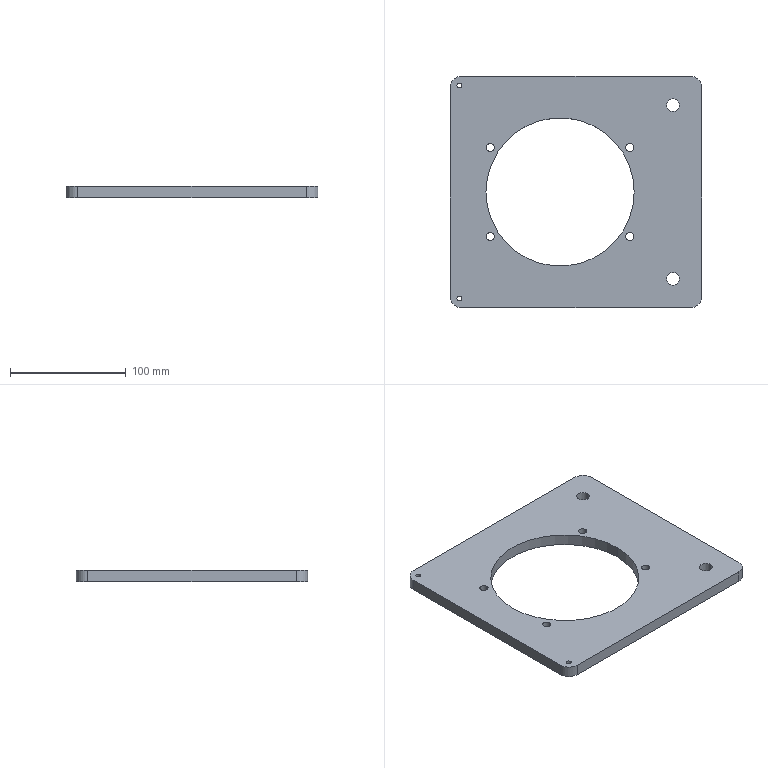Part | SolidWorks | features ICE 3, Cut 2, Extrusion 1, Fillet 1, HoleWzd 1 | 1 solid | 28 faces | box 217.5 x 200 x 10 mm | volume 301745 mm3 | cylinder 22 | plane 6 | commonest cylinder face diameters 7 x8 4.2 x4 11 x4 20 x4 128 x2
STEP:
#1=CARTESIAN_POINT('',(-84.9,92.,0.));
#2=VERTEX_POINT('',#1);
#3=CARTESIAN_POINT('',(-89.1,92.,0.));
#4=VERTEX_POINT('',#3);
#5=CARTESIAN_POINT('',(-87.,92.,0.));
#6=DIRECTION('',(0.,0.,-1.));
#7=DIRECTION('',(-1.,0.,0.));
#8=AXIS2_PLACEMENT_3D('',#5,#6,#7);
#9=CIRCLE('',#8,2.1);
#10=EDGE_CURVE('',#2,#4,#9,.T.);
#11=ORIENTED_EDGE('',*,*,#10,.T.);
#12=CARTESIAN_POINT('',(-89.1,92.,10.));
#13=VERTEX_POINT('',#12);
#14=CARTESIAN_POINT('',(-89.1,92.,10.));
#15=DIRECTION('',(0.,0.,1.));
#16=VECTOR('',#15,1000.);
#17=LINE('',#14,#16);
#18=EDGE_CURVE('',#4,#13,#17,.T.);
#19=ORIENTED_EDGE('',*,*,#18,.T.);
#20=CARTESIAN_POINT('',(-84.9,92.,10.));
#21=VERTEX_POINT('',#20);
#22=CARTESIAN_POINT('',(-87.,92.,10.));
#23=DIRECTION('',(0.,0.,1.));
#24=DIRECTION('',(1.,0.,0.));
#25=AXIS2_PLACEMENT_3D('',#22,#23,#24);
#26=CIRCLE('',#25,2.1);
#27=EDGE_CURVE('',#13,#21,#26,.T.);
#28=ORIENTED_EDGE('',*,*,#27,.T.);
#29=CARTESIAN_POINT('',(-84.9,92.,10.));
#30=DIRECTION('',(0.,0.,1.));
#31=VECTOR('',#30,1000.);
#32=LINE('',#29,#31);
#33=EDGE_CURVE('',#2,#21,#32,.T.);
#34=ORIENTED_EDGE('',*,*,#33,.F.);
#35=EDGE_LOOP('',(#11,#19,#28,#34));
#36=FACE_OUTER_BOUND('',#35,.T.);
#37=CARTESIAN_POINT('',(-87.,92.,10.));
#38=DIRECTION('',(0.,0.,1.));
#39=DIRECTION('',(1.,0.,0.));
#40=AXIS2_PLACEMENT_3D('',#37,#38,#39);
#41=CYLINDRICAL_SURFACE('',#40,2.1);
#42=ADVANCED_FACE('',(#36),#41,.F.);
#43=CARTESIAN_POINT('',(-84.9,-92.,0.));
#44=VERTEX_POINT('',#43);
#45=CARTESIAN_POINT('',(-89.1,-92.,0.));
#46=VERTEX_POINT('',#45);
#47=CARTESIAN_POINT('',(-87.,-92.,0.));
#48=DIRECTION('',(0.,0.,-1.));
#49=DIRECTION('',(-1.,0.,0.));
#50=AXIS2_PLACEMENT_3D('',#47,#48,#49);
#51=CIRCLE('',#50,2.1);
#52=EDGE_CURVE('',#44,#46,#51,.T.);
#53=ORIENTED_EDGE('',*,*,#52,.T.);
#54=CARTESIAN_POINT('',(-89.1,-92.,10.));
#55=VERTEX_POINT('',#54);
#56=CARTESIAN_POINT('',(-89.1,-92.,10.));
#57=DIRECTION('',(0.,0.,1.));
#58=VECTOR('',#57,1000.);
#59=LINE('',#56,#58);
#60=EDGE_CURVE('',#46,#55,#59,.T.);
#61=ORIENTED_EDGE('',*,*,#60,.T.);
#62=CARTESIAN_POINT('',(-84.9,-92.,10.));
#63=VERTEX_POINT('',#62);
#64=CARTESIAN_POINT('',(-87.,-92.,10.));
#65=DIRECTION('',(0.,0.,1.));
#66=DIRECTION('',(1.,0.,0.));
#67=AXIS2_PLACEMENT_3D('',#64,#65,#66);
#68=CIRCLE('',#67,2.1);
#69=EDGE_CURVE('',#55,#63,#68,.T.);
#70=ORIENTED_EDGE('',*,*,#69,.T.);
#71=CARTESIAN_POINT('',(-84.9,-92.,10.));
#72=DIRECTION('',(0.,0.,1.));
#73=VECTOR('',#72,1000.);
#74=LINE('',#71,#73);
#75=EDGE_CURVE('',#44,#63,#74,.T.);
#76=ORIENTED_EDGE('',*,*,#75,.F.);
#77=EDGE_LOOP('',(#53,#61,#70,#76));
#78=FACE_OUTER_BOUND('',#77,.T.);
#79=CARTESIAN_POINT('',(-87.,-92.,10.));
#80=DIRECTION('',(0.,0.,1.));
#81=DIRECTION('',(1.,0.,0.));
#82=AXIS2_PLACEMENT_3D('',#79,#80,#81);
#83=CYLINDRICAL_SURFACE('',#82,2.1);
#84=ADVANCED_FACE('',(#78),#83,.F.);
#85=CARTESIAN_POINT('',(92.,-75.,0.));
#86=VERTEX_POINT('',#85);
#87=CARTESIAN_POINT('',(103.,-75.,0.));
#88=VERTEX_POINT('',#87);
#89=CARTESIAN_POINT('',(97.5,-75.,0.));
#90=DIRECTION('',(0.,0.,1.));
#91=DIRECTION('',(-1.,0.,0.));
#92=AXIS2_PLACEMENT_3D('',#89,#90,#91);
#93=CIRCLE('',#92,5.5);
#94=EDGE_CURVE('',#86,#88,#93,.T.);
#95=ORIENTED_EDGE('',*,*,#94,.F.);
#96=CARTESIAN_POINT('',(92.,-75.,10.));
#97=VERTEX_POINT('',#96);
#98=CARTESIAN_POINT('',(92.,-75.,0.));
#99=DIRECTION('',(0.,0.,1.));
#100=VECTOR('',#99,1000.);
#101=LINE('',#98,#100);
#102=EDGE_CURVE('',#86,#97,#101,.T.);
#103=ORIENTED_EDGE('',*,*,#102,.T.);
#104=CARTESIAN_POINT('',(103.,-75.,10.));
#105=VERTEX_POINT('',#104);
#106=CARTESIAN_POINT('',(97.5,-75.,10.));
#107=DIRECTION('',(0.,0.,1.));
#108=DIRECTION('',(-1.,0.,0.));
#109=AXIS2_PLACEMENT_3D('',#106,#107,#108);
#110=CIRCLE('',#109,5.5);
#111=EDGE_CURVE('',#97,#105,#110,.T.);
#112=ORIENTED_EDGE('',*,*,#111,.T.);
#113=CARTESIAN_POINT('',(103.,-75.,0.));
#114=DIRECTION('',(0.,0.,1.));
#115=VECTOR('',#114,1000.);
#116=LINE('',#113,#115);
#117=EDGE_CURVE('',#88,#105,#116,.T.);
#118=ORIENTED_EDGE('',*,*,#117,.F.);
#119=EDGE_LOOP('',(#95,#103,#112,#118));
#120=FACE_OUTER_BOUND('',#119,.T.);
#121=CARTESIAN_POINT('',(97.5,-75.,0.));
#122=DIRECTION('',(0.,0.,1.));
#123=DIRECTION('',(1.,0.,0.));
#124=AXIS2_PLACEMENT_3D('',#121,#122,#123);
#125=CYLINDRICAL_SURFACE('',#124,5.5);
#126=ADVANCED_FACE('',(#120),#125,.F.);
#127=CARTESIAN_POINT('',(92.,75.,0.));
#128=VERTEX_POINT('',#127);
#129=CARTESIAN_POINT('',(103.,75.,0.));
#130=VERTEX_POINT('',#129);
#131=CARTESIAN_POINT('',(97.5,75.,0.));
#132=DIRECTION('',(0.,0.,1.));
#133=DIRECTION('',(1.,0.,0.));
#134=AXIS2_PLACEMENT_3D('',#131,#132,#133);
#135=CIRCLE('',#134,5.5);
#136=EDGE_CURVE('',#128,#130,#135,.T.);
#137=ORIENTED_EDGE('',*,*,#136,.F.);
#138=CARTESIAN_POINT('',(92.,75.,10.));
#139=VERTEX_POINT('',#138);
#140=CARTESIAN_POINT('',(92.,75.,0.));
#141=DIRECTION('',(0.,0.,1.));
#142=VECTOR('',#141,1000.);
#143=LINE('',#140,#142);
#144=EDGE_CURVE('',#128,#139,#143,.T.);
#145=ORIENTED_EDGE('',*,*,#144,.T.);
#146=CARTESIAN_POINT('',(103.,75.,10.));
#147=VERTEX_POINT('',#146);
#148=CARTESIAN_POINT('',(97.5,75.,10.));
#149=DIRECTION('',(0.,0.,1.));
#150=DIRECTION('',(1.,0.,0.));
#151=AXIS2_PLACEMENT_3D('',#148,#149,#150);
#152=CIRCLE('',#151,5.5);
#153=EDGE_CURVE('',#139,#147,#152,.T.);
#154=ORIENTED_EDGE('',*,*,#153,.T.);
#155=CARTESIAN_POINT('',(103.,75.,0.));
#156=DIRECTION('',(0.,0.,1.));
#157=VECTOR('',#156,1000.);
#158=LINE('',#155,#157);
#159=EDGE_CURVE('',#130,#147,#158,.T.);
#160=ORIENTED_EDGE('',*,*,#159,.F.);
#161=EDGE_LOOP('',(#137,#145,#154,#160));
#162=FACE_OUTER_BOUND('',#161,.T.);
#163=CARTESIAN_POINT('',(97.5,75.,0.));
#164=DIRECTION('',(0.,0.,1.));
#165=DIRECTION('',(1.,0.,0.));
#166=AXIS2_PLACEMENT_3D('',#163,#164,#165);
#167=CYLINDRICAL_SURFACE('',#166,5.5);
#168=ADVANCED_FACE('',(#162),#167,.F.);
#169=CARTESIAN_POINT('',(56.75,38.425,0.));
#170=VERTEX_POINT('',#169);
#171=CARTESIAN_POINT('',(63.75,38.425,0.));
#172=VERTEX_POINT('',#171);
#173=CARTESIAN_POINT('',(60.25,38.425,0.));
#174=DIRECTION('',(0.,0.,1.));
#175=DIRECTION('',(-1.,0.,0.));
#176=AXIS2_PLACEMENT_3D('',#173,#174,#175);
#177=CIRCLE('',#176,3.5);
#178=EDGE_CURVE('',#170,#172,#177,.T.);
#179=ORIENTED_EDGE('',*,*,#178,.F.);
#180=CARTESIAN_POINT('',(56.75,38.425,10.));
#181=VERTEX_POINT('',#180);
#182=CARTESIAN_POINT('',(56.75,38.425,0.));
#183=DIRECTION('',(0.,0.,1.));
#184=VECTOR('',#183,1000.);
#185=LINE('',#182,#184);
#186=EDGE_CURVE('',#170,#181,#185,.T.);
#187=ORIENTED_EDGE('',*,*,#186,.T.);
#188=CARTESIAN_POINT('',(63.75,38.425,10.));
#189=VERTEX_POINT('',#188);
#190=CARTESIAN_POINT('',(60.25,38.425,10.));
#191=DIRECTION('',(0.,0.,1.));
#192=DIRECTION('',(-1.,0.,0.));
#193=AXIS2_PLACEMENT_3D('',#190,#191,#192);
#194=CIRCLE('',#193,3.5);
#195=EDGE_CURVE('',#181,#189,#194,.T.);
#196=ORIENTED_EDGE('',*,*,#195,.T.);
#197=CARTESIAN_POINT('',(63.75,38.425,0.));
#198=DIRECTION('',(0.,0.,1.));
#199=VECTOR('',#198,1000.);
#200=LINE('',#197,#199);
#201=EDGE_CURVE('',#172,#189,#200,.T.);
#202=ORIENTED_EDGE('',*,*,#201,.F.);
#203=EDGE_LOOP('',(#179,#187,#196,#202));
#204=FACE_OUTER_BOUND('',#203,.T.);
#205=CARTESIAN_POINT('',(60.25,38.425,0.));
#206=DIRECTION('',(0.,0.,1.));
#207=DIRECTION('',(1.,0.,0.));
#208=AXIS2_PLACEMENT_3D('',#205,#206,#207);
#209=CYLINDRICAL_SURFACE('',#208,3.5);
#210=ADVANCED_FACE('',(#204),#209,.F.);
#211=CARTESIAN_POINT('',(56.75,-38.425,0.));
#212=VERTEX_POINT('',#211);
#213=CARTESIAN_POINT('',(63.75,-38.425,0.));
#214=VERTEX_POINT('',#213);
#215=CARTESIAN_POINT('',(60.25,-38.425,0.));
#216=DIRECTION('',(0.,0.,1.));
#217=DIRECTION('',(1.,0.,0.));
#218=AXIS2_PLACEMENT_3D('',#215,#216,#217);
#219=CIRCLE('',#218,3.5);
#220=EDGE_CURVE('',#212,#214,#219,.T.);
#221=ORIENTED_EDGE('',*,*,#220,.F.);
#222=CARTESIAN_POINT('',(56.75,-38.425,10.));
#223=VERTEX_POINT('',#222);
#224=CARTESIAN_POINT('',(56.75,-38.425,0.));
#225=DIRECTION('',(0.,0.,1.));
#226=VECTOR('',#225,1000.);
#227=LINE('',#224,#226);
#228=EDGE_CURVE('',#212,#223,#227,.T.);
#229=ORIENTED_EDGE('',*,*,#228,.T.);
#230=CARTESIAN_POINT('',(63.75,-38.425,10.));
#231=VERTEX_POINT('',#230);
#232=CARTESIAN_POINT('',(60.25,-38.425,10.));
#233=DIRECTION('',(0.,0.,1.));
#234=DIRECTION('',(1.,0.,0.));
#235=AXIS2_PLACEMENT_3D('',#232,#233,#234);
#236=CIRCLE('',#235,3.5);
#237=EDGE_CURVE('',#223,#231,#236,.T.);
#238=ORIENTED_EDGE('',*,*,#237,.T.);
#239=CARTESIAN_POINT('',(63.75,-38.425,0.));
#240=DIRECTION('',(0.,0.,1.));
#241=VECTOR('',#240,1000.);
#242=LINE('',#239,#241);
#243=EDGE_CURVE('',#214,#231,#242,.T.);
#244=ORIENTED_EDGE('',*,*,#243,.F.);
#245=EDGE_LOOP('',(#221,#229,#238,#244));
#246=FACE_OUTER_BOUND('',#245,.T.);
#247=CARTESIAN_POINT('',(60.25,-38.425,0.));
#248=DIRECTION('',(0.,0.,1.));
#249=DIRECTION('',(1.,0.,0.));
#250=AXIS2_PLACEMENT_3D('',#247,#248,#249);
#251=CYLINDRICAL_SURFACE('',#250,3.5);
#252=ADVANCED_FACE('',(#246),#251,.F.);
#253=CARTESIAN_POINT('',(-63.75,-38.425,0.));
#254=VERTEX_POINT('',#253);
#255=CARTESIAN_POINT('',(-56.75,-38.425,0.));
#256=VERTEX_POINT('',#255);
#257=CARTESIAN_POINT('',(-60.25,-38.425,0.));
#258=DIRECTION('',(0.,0.,1.));
#259=DIRECTION('',(-1.,0.,0.));
#260=AXIS2_PLACEMENT_3D('',#257,#258,#259);
#261=CIRCLE('',#260,3.5);
#262=EDGE_CURVE('',#254,#256,#261,.T.);
#263=ORIENTED_EDGE('',*,*,#262,.F.);
#264=CARTESIAN_POINT('',(-63.75,-38.425,10.));
#265=VERTEX_POINT('',#264);
#266=CARTESIAN_POINT('',(-63.75,-38.425,0.));
#267=DIRECTION('',(0.,0.,1.));
#268=VECTOR('',#267,1000.);
#269=LINE('',#266,#268);
#270=EDGE_CURVE('',#254,#265,#269,.T.);
#271=ORIENTED_EDGE('',*,*,#270,.T.);
#272=CARTESIAN_POINT('',(-56.75,-38.425,10.));
#273=VERTEX_POINT('',#272);
#274=CARTESIAN_POINT('',(-60.25,-38.425,10.));
#275=DIRECTION('',(0.,0.,1.));
#276=DIRECTION('',(-1.,0.,0.));
#277=AXIS2_PLACEMENT_3D('',#274,#275,#276);
#278=CIRCLE('',#277,3.5);
#279=EDGE_CURVE('',#265,#273,#278,.T.);
#280=ORIENTED_EDGE('',*,*,#279,.T.);
#281=CARTESIAN_POINT('',(-56.75,-38.425,0.));
#282=DIRECTION('',(0.,0.,1.));
#283=VECTOR('',#282,1000.);
#284=LINE('',#281,#283);
#285=EDGE_CURVE('',#256,#273,#284,.T.);
#286=ORIENTED_EDGE('',*,*,#285,.F.);
#287=EDGE_LOOP('',(#263,#271,#280,#286));
#288=FACE_OUTER_BOUND('',#287,.T.);
#289=CARTESIAN_POINT('',(-60.25,-38.425,0.));
#290=DIRECTION('',(0.,0.,1.));
#291=DIRECTION('',(1.,0.,0.));
#292=AXIS2_PLACEMENT_3D('',#289,#290,#291);
#293=CYLINDRICAL_SURFACE('',#292,3.5);
#294=ADVANCED_FACE('',(#288),#293,.F.);
#295=CARTESIAN_POINT('',(-63.75,38.425,0.));
#296=VERTEX_POINT('',#295);
#297=CARTESIAN_POINT('',(-56.75,38.425,0.));
#298=VERTEX_POINT('',#297);
#299=CARTESIAN_POINT('',(-60.25,38.425,0.));
#300=DIRECTION('',(0.,0.,1.));
#301=DIRECTION('',(1.,0.,0.));
#302=AXIS2_PLACEMENT_3D('',#299,#300,#301);
#303=CIRCLE('',#302,3.5);
#304=EDGE_CURVE('',#296,#298,#303,.T.);
#305=ORIENTED_EDGE('',*,*,#304,.F.);
#306=CARTESIAN_POINT('',(-63.75,38.425,10.));
#307=VERTEX_POINT('',#306);
#308=CARTESIAN_POINT('',(-63.75,38.425,0.));
#309=DIRECTION('',(0.,0.,1.));
#310=VECTOR('',#309,1000.);
#311=LINE('',#308,#310);
#312=EDGE_CURVE('',#296,#307,#311,.T.);
#313=ORIENTED_EDGE('',*,*,#312,.T.);
#314=CARTESIAN_POINT('',(-56.75,38.425,10.));
#315=VERTEX_POINT('',#314);
#316=CARTESIAN_POINT('',(-60.25,38.425,10.));
#317=DIRECTION('',(0.,0.,1.));
#318=DIRECTION('',(1.,0.,0.));
#319=AXIS2_PLACEMENT_3D('',#316,#317,#318);
#320=CIRCLE('',#319,3.5);
#321=EDGE_CURVE('',#307,#315,#320,.T.);
#322=ORIENTED_EDGE('',*,*,#321,.T.);
#323=CARTESIAN_POINT('',(-56.75,38.425,0.));
#324=DIRECTION('',(0.,0.,1.));
#325=VECTOR('',#324,1000.);
#326=LINE('',#323,#325);
#327=EDGE_CURVE('',#298,#315,#326,.T.);
#328=ORIENTED_EDGE('',*,*,#327,.F.);
#329=EDGE_LOOP('',(#305,#313,#322,#328));
#330=FACE_OUTER_BOUND('',#329,.T.);
#331=CARTESIAN_POINT('',(-60.25,38.425,0.));
#332=DIRECTION('',(0.,0.,1.));
#333=DIRECTION('',(1.,0.,0.));
#334=AXIS2_PLACEMENT_3D('',#331,#332,#333);
#335=CYLINDRICAL_SURFACE('',#334,3.5);
#336=ADVANCED_FACE('',(#330),#335,.F.);
#337=CARTESIAN_POINT('',(-64.,0.,0.));
#338=VERTEX_POINT('',#337);
#339=CARTESIAN_POINT('',(64.,0.,0.));
#340=VERTEX_POINT('',#339);
#341=CARTESIAN_POINT('',(0.,0.,0.));
#342=DIRECTION('',(0.,0.,1.));
#343=DIRECTION('',(-1.,0.,0.));
#344=AXIS2_PLACEMENT_3D('',#341,#342,#343);
#345=CIRCLE('',#344,64.);
#346=EDGE_CURVE('',#338,#340,#345,.T.);
#347=ORIENTED_EDGE('',*,*,#346,.F.);
#348=CARTESIAN_POINT('',(-64.,0.,10.));
#349=VERTEX_POINT('',#348);
#350=CARTESIAN_POINT('',(-64.,0.,-181.019));
#351=DIRECTION('',(0.,0.,1.));
#352=VECTOR('',#351,1000.);
#353=LINE('',#350,#352);
#354=EDGE_CURVE('',#338,#349,#353,.T.);
#355=ORIENTED_EDGE('',*,*,#354,.T.);
#356=CARTESIAN_POINT('',(64.,0.,10.));
#357=VERTEX_POINT('',#356);
#358=CARTESIAN_POINT('',(0.,0.,10.));
#359=DIRECTION('',(0.,0.,1.));
#360=DIRECTION('',(1.,0.,0.));
#361=AXIS2_PLACEMENT_3D('',#358,#359,#360);
#362=CIRCLE('',#361,64.);
#363=EDGE_CURVE('',#349,#357,#362,.T.);
#364=ORIENTED_EDGE('',*,*,#363,.T.);
#365=CARTESIAN_POINT('',(64.,0.,-181.019));
#366=DIRECTION('',(0.,0.,1.));
#367=VECTOR('',#366,1000.);
#368=LINE('',#365,#367);
#369=EDGE_CURVE('',#340,#357,#368,.T.);
#370=ORIENTED_EDGE('',*,*,#369,.F.);
#371=EDGE_LOOP('',(#347,#355,#364,#370));
#372=FACE_OUTER_BOUND('',#371,.T.);
#373=CARTESIAN_POINT('',(0.,0.,-181.019));
#374=DIRECTION('',(0.,0.,1.));
#375=DIRECTION('',(1.,0.,0.));
#376=AXIS2_PLACEMENT_3D('',#373,#374,#375);
#377=CYLINDRICAL_SURFACE('',#376,64.);
#378=ADVANCED_FACE('',(#372),#377,.F.);
#379=CARTESIAN_POINT('',(-87.,92.,10.));
#380=DIRECTION('',(0.,0.,1.));
#381=DIRECTION('',(1.,0.,0.));
#382=AXIS2_PLACEMENT_3D('',#379,#380,#381);
#383=CIRCLE('',#382,2.1);
#384=EDGE_CURVE('',#21,#13,#383,.T.);
#385=ORIENTED_EDGE('',*,*,#384,.F.);
#386=ORIENTED_EDGE('',*,*,#27,.F.);
#387=EDGE_LOOP('',(#385,#386));
#388=FACE_BOUND('',#387,.T.);
#389=CARTESIAN_POINT('',(-95.,90.,10.));
#390=VERTEX_POINT('',#389);
#391=CARTESIAN_POINT('',(-95.,-90.,10.));
#392=VERTEX_POINT('',#391);
#393=CARTESIAN_POINT('',(-95.,-100.,10.));
#394=DIRECTION('',(0.,-1.,0.));
#395=VECTOR('',#394,1000.);
#396=LINE('',#393,#395);
#397=EDGE_CURVE('',#390,#392,#396,.T.);
#398=ORIENTED_EDGE('',*,*,#397,.T.);
#399=CARTESIAN_POINT('',(-85.,-100.,10.));
#400=VERTEX_POINT('',#399);
#401=CARTESIAN_POINT('',(-85.,-90.,10.));
#402=DIRECTION('',(0.,0.,1.));
#403=DIRECTION('',(-1.,0.,0.));
#404=AXIS2_PLACEMENT_3D('',#401,#402,#403);
#405=CIRCLE('',#404,10.);
#406=EDGE_CURVE('',#392,#400,#405,.T.);
#407=ORIENTED_EDGE('',*,*,#406,.T.);
#408=CARTESIAN_POINT('',(112.5,-100.,10.));
#409=VERTEX_POINT('',#408);
#410=CARTESIAN_POINT('',(-95.,-100.,10.));
#411=DIRECTION('',(1.,0.,0.));
#412=VECTOR('',#411,1000.);
#413=LINE('',#410,#412);
#414=EDGE_CURVE('',#400,#409,#413,.T.);
#415=ORIENTED_EDGE('',*,*,#414,.T.);
#416=CARTESIAN_POINT('',(122.5,-90.,10.));
#417=VERTEX_POINT('',#416);
#418=CARTESIAN_POINT('',(112.5,-90.,10.));
#419=DIRECTION('',(0.,0.,1.));
#420=DIRECTION('',(-1.,0.,0.));
#421=AXIS2_PLACEMENT_3D('',#418,#419,#420);
#422=CIRCLE('',#421,10.);
#423=EDGE_CURVE('',#409,#417,#422,.T.);
#424=ORIENTED_EDGE('',*,*,#423,.T.);
#425=CARTESIAN_POINT('',(122.5,90.,10.));
#426=VERTEX_POINT('',#425);
#427=CARTESIAN_POINT('',(122.5,-100.,10.));
#428=DIRECTION('',(0.,1.,0.));
#429=VECTOR('',#428,1000.);
#430=LINE('',#427,#429);
#431=EDGE_CURVE('',#417,#426,#430,.T.);
#432=ORIENTED_EDGE('',*,*,#431,.T.);
#433=CARTESIAN_POINT('',(112.5,100.,10.));
#434=VERTEX_POINT('',#433);
#435=CARTESIAN_POINT('',(112.5,90.,10.));
#436=DIRECTION('',(0.,0.,1.));
#437=DIRECTION('',(-1.,0.,0.));
#438=AXIS2_PLACEMENT_3D('',#435,#436,#437);
#439=CIRCLE('',#438,10.);
#440=EDGE_CURVE('',#426,#434,#439,.T.);
#441=ORIENTED_EDGE('',*,*,#440,.T.);
#442=CARTESIAN_POINT('',(-85.,100.,10.));
#443=VERTEX_POINT('',#442);
#444=CARTESIAN_POINT('',(-95.,100.,10.));
#445=DIRECTION('',(-1.,0.,0.));
#446=VECTOR('',#445,1000.);
#447=LINE('',#444,#446);
#448=EDGE_CURVE('',#434,#443,#447,.T.);
#449=ORIENTED_EDGE('',*,*,#448,.T.);
#450=CARTESIAN_POINT('',(-85.,90.,10.));
#451=DIRECTION('',(0.,0.,1.));
#452=DIRECTION('',(-1.,0.,0.));
#453=AXIS2_PLACEMENT_3D('',#450,#451,#452);
#454=CIRCLE('',#453,10.);
#455=EDGE_CURVE('',#443,#390,#454,.T.);
#456=ORIENTED_EDGE('',*,*,#455,.T.);
#457=EDGE_LOOP('',(#398,#407,#415,#424,#432,#441,#449,#456));
#458=FACE_OUTER_BOUND('',#457,.T.);
#459=CARTESIAN_POINT('',(0.,0.,10.));
#460=DIRECTION('',(0.,0.,1.));
#461=DIRECTION('',(1.,0.,0.));
#462=AXIS2_PLACEMENT_3D('',#459,#460,#461);
#463=CIRCLE('',#462,64.);
#464=EDGE_CURVE('',#357,#349,#463,.T.);
#465=ORIENTED_EDGE('',*,*,#464,.F.);
#466=ORIENTED_EDGE('',*,*,#363,.F.);
#467=EDGE_LOOP('',(#465,#466));
#468=FACE_BOUND('',#467,.T.);
#469=CARTESIAN_POINT('',(-60.25,38.425,10.));
#470=DIRECTION('',(0.,0.,1.));
#471=DIRECTION('',(1.,0.,0.));
#472=AXIS2_PLACEMENT_3D('',#469,#470,#471);
#473=CIRCLE('',#472,3.5);
#474=EDGE_CURVE('',#315,#307,#473,.T.);
#475=ORIENTED_EDGE('',*,*,#474,.F.);
#476=ORIENTED_EDGE('',*,*,#321,.F.);
#477=EDGE_LOOP('',(#475,#476));
#478=FACE_BOUND('',#477,.T.);
#479=CARTESIAN_POINT('',(-60.25,-38.425,10.));
#480=DIRECTION('',(0.,0.,1.));
#481=DIRECTION('',(-1.,0.,0.));
#482=AXIS2_PLACEMENT_3D('',#479,#480,#481);
#483=CIRCLE('',#482,3.5);
#484=EDGE_CURVE('',#273,#265,#483,.T.);
#485=ORIENTED_EDGE('',*,*,#484,.F.);
#486=ORIENTED_EDGE('',*,*,#279,.F.);
#487=EDGE_LOOP('',(#485,#486));
#488=FACE_BOUND('',#487,.T.);
#489=CARTESIAN_POINT('',(60.25,-38.425,10.));
#490=DIRECTION('',(0.,0.,1.));
#491=DIRECTION('',(1.,0.,0.));
#492=AXIS2_PLACEMENT_3D('',#489,#490,#491);
#493=CIRCLE('',#492,3.5);
#494=EDGE_CURVE('',#231,#223,#493,.T.);
#495=ORIENTED_EDGE('',*,*,#494,.F.);
#496=ORIENTED_EDGE('',*,*,#237,.F.);
#497=EDGE_LOOP('',(#495,#496));
#498=FACE_BOUND('',#497,.T.);
#499=CARTESIAN_POINT('',(60.25,38.425,10.));
#500=DIRECTION('',(0.,0.,1.));
#501=DIRECTION('',(-1.,0.,0.));
#502=AXIS2_PLACEMENT_3D('',#499,#500,#501);
#503=CIRCLE('',#502,3.5);
#504=EDGE_CURVE('',#189,#181,#503,.T.);
#505=ORIENTED_EDGE('',*,*,#504,.F.);
#506=ORIENTED_EDGE('',*,*,#195,.F.);
#507=EDGE_LOOP('',(#505,#506));
#508=FACE_BOUND('',#507,.T.);
#509=CARTESIAN_POINT('',(97.5,75.,10.));
#510=DIRECTION('',(0.,0.,1.));
#511=DIRECTION('',(1.,0.,0.));
#512=AXIS2_PLACEMENT_3D('',#509,#510,#511);
#513=CIRCLE('',#512,5.5);
#514=EDGE_CURVE('',#147,#139,#513,.T.);
#515=ORIENTED_EDGE('',*,*,#514,.F.);
#516=ORIENTED_EDGE('',*,*,#153,.F.);
#517=EDGE_LOOP('',(#515,#516));
#518=FACE_BOUND('',#517,.T.);
#519=CARTESIAN_POINT('',(97.5,-75.,10.));
#520=DIRECTION('',(0.,0.,1.));
#521=DIRECTION('',(-1.,0.,0.));
#522=AXIS2_PLACEMENT_3D('',#519,#520,#521);
#523=CIRCLE('',#522,5.5);
#524=EDGE_CURVE('',#105,#97,#523,.T.);
#525=ORIENTED_EDGE('',*,*,#524,.F.);
#526=ORIENTED_EDGE('',*,*,#111,.F.);
#527=EDGE_LOOP('',(#525,#526));
#528=FACE_BOUND('',#527,.T.);
#529=CARTESIAN_POINT('',(-87.,-92.,10.));
#530=DIRECTION('',(0.,0.,1.));
#531=DIRECTION('',(1.,0.,0.));
#532=AXIS2_PLACEMENT_3D('',#529,#530,#531);
#533=CIRCLE('',#532,2.1);
#534=EDGE_CURVE('',#63,#55,#533,.T.);
#535=ORIENTED_EDGE('',*,*,#534,.F.);
#536=ORIENTED_EDGE('',*,*,#69,.F.);
#537=EDGE_LOOP('',(#535,#536));
#538=FACE_BOUND('',#537,.T.);
#539=CARTESIAN_POINT('',(0.,0.,10.));
#540=DIRECTION('',(0.,0.,-1.));
#541=DIRECTION('',(-1.,0.,0.));
#542=AXIS2_PLACEMENT_3D('',#539,#540,#541);
#543=PLANE('',#542);
#544=ADVANCED_FACE('',(#388,#458,#468,#478,#488,#498,#508,#518,#528,#538),#543,.F.);
#545=ORIENTED_EDGE('',*,*,#448,.F.);
#546=CARTESIAN_POINT('',(112.5,100.,0.));
#547=VERTEX_POINT('',#546);
#548=CARTESIAN_POINT('',(112.5,100.,0.));
#549=DIRECTION('',(0.,0.,-1.));
#550=VECTOR('',#549,1000.);
#551=LINE('',#548,#550);
#552=EDGE_CURVE('',#434,#547,#551,.T.);
#553=ORIENTED_EDGE('',*,*,#552,.T.);
#554=CARTESIAN_POINT('',(-85.,100.,0.));
#555=VERTEX_POINT('',#554);
#556=CARTESIAN_POINT('',(-95.,100.,0.));
#557=DIRECTION('',(-1.,0.,0.));
#558=VECTOR('',#557,1000.);
#559=LINE('',#556,#558);
#560=EDGE_CURVE('',#547,#555,#559,.T.);
#561=ORIENTED_EDGE('',*,*,#560,.T.);
#562=CARTESIAN_POINT('',(-85.,100.,10.));
#563=DIRECTION('',(0.,0.,1.));
#564=VECTOR('',#563,1000.);
#565=LINE('',#562,#564);
#566=EDGE_CURVE('',#555,#443,#565,.T.);
#567=ORIENTED_EDGE('',*,*,#566,.T.);
#568=EDGE_LOOP('',(#545,#553,#561,#567));
#569=FACE_OUTER_BOUND('',#568,.T.);
#570=CARTESIAN_POINT('',(-95.,100.,10.));
#571=DIRECTION('',(0.,-1.,0.));
#572=DIRECTION('',(0.,0.,-1.));
#573=AXIS2_PLACEMENT_3D('',#570,#571,#572);
#574=PLANE('',#573);
#575=ADVANCED_FACE('',(#569),#574,.F.);
#576=CARTESIAN_POINT('',(-95.,90.,0.));
#577=VERTEX_POINT('',#576);
#578=CARTESIAN_POINT('',(-95.,-90.,0.));
#579=VERTEX_POINT('',#578);
#580=CARTESIAN_POINT('',(-95.,-100.,0.));
#581=DIRECTION('',(0.,-1.,0.));
#582=VECTOR('',#581,1000.);
#583=LINE('',#580,#582);
#584=EDGE_CURVE('',#577,#579,#583,.T.);
#585=ORIENTED_EDGE('',*,*,#584,.T.);
#586=CARTESIAN_POINT('',(-95.,-90.,10.));
#587=DIRECTION('',(0.,0.,1.));
#588=VECTOR('',#587,1000.);
#589=LINE('',#586,#588);
#590=EDGE_CURVE('',#579,#392,#589,.T.);
#591=ORIENTED_EDGE('',*,*,#590,.T.);
#592=ORIENTED_EDGE('',*,*,#397,.F.);
#593=CARTESIAN_POINT('',(-95.,90.,10.));
#594=DIRECTION('',(0.,0.,-1.));
#595=VECTOR('',#594,1000.);
#596=LINE('',#593,#595);
#597=EDGE_CURVE('',#390,#577,#596,.T.);
#598=ORIENTED_EDGE('',*,*,#597,.T.);
#599=EDGE_LOOP('',(#585,#591,#592,#598));
#600=FACE_OUTER_BOUND('',#599,.T.);
#601=CARTESIAN_POINT('',(-95.,-100.,10.));
#602=DIRECTION('',(1.,0.,0.));
#603=DIRECTION('',(0.,0.,-1.));
#604=AXIS2_PLACEMENT_3D('',#601,#602,#603);
#605=PLANE('',#604);
#606=ADVANCED_FACE('',(#600),#605,.F.);
#607=ORIENTED_EDGE('',*,*,#414,.F.);
#608=CARTESIAN_POINT('',(-85.,-100.,0.));
#609=VERTEX_POINT('',#608);
#610=CARTESIAN_POINT('',(-85.,-100.,10.));
#611=DIRECTION('',(0.,0.,-1.));
#612=VECTOR('',#611,1000.);
#613=LINE('',#610,#612);
#614=EDGE_CURVE('',#400,#609,#613,.T.);
#615=ORIENTED_EDGE('',*,*,#614,.T.);
#616=CARTESIAN_POINT('',(112.5,-100.,0.));
#617=VERTEX_POINT('',#616);
#618=CARTESIAN_POINT('',(-95.,-100.,0.));
#619=DIRECTION('',(1.,0.,0.));
#620=VECTOR('',#619,1000.);
#621=LINE('',#618,#620);
#622=EDGE_CURVE('',#609,#617,#621,.T.);
#623=ORIENTED_EDGE('',*,*,#622,.T.);
#624=CARTESIAN_POINT('',(112.5,-100.,10.));
#625=DIRECTION('',(0.,0.,1.));
#626=VECTOR('',#625,1000.);
#627=LINE('',#624,#626);
#628=EDGE_CURVE('',#617,#409,#627,.T.);
#629=ORIENTED_EDGE('',*,*,#628,.T.);
#630=EDGE_LOOP('',(#607,#615,#623,#629));
#631=FACE_OUTER_BOUND('',#630,.T.);
#632=CARTESIAN_POINT('',(-95.,-100.,10.));
#633=DIRECTION('',(0.,1.,0.));
#634=DIRECTION('',(0.,0.,1.));
#635=AXIS2_PLACEMENT_3D('',#632,#633,#634);
#636=PLANE('',#635);
#637=ADVANCED_FACE('',(#631),#636,.F.);
#638=ORIENTED_EDGE('',*,*,#10,.F.);
#639=CARTESIAN_POINT('',(-87.,92.,0.));
#640=DIRECTION('',(0.,0.,-1.));
#641=DIRECTION('',(-1.,0.,0.));
#642=AXIS2_PLACEMENT_3D('',#639,#640,#641);
#643=CIRCLE('',#642,2.1);
#644=EDGE_CURVE('',#4,#2,#643,.T.);
#645=ORIENTED_EDGE('',*,*,#644,.F.);
#646=EDGE_LOOP('',(#638,#645));
#647=FACE_BOUND('',#646,.T.);
#648=ORIENTED_EDGE('',*,*,#52,.F.);
#649=CARTESIAN_POINT('',(-87.,-92.,0.));
#650=DIRECTION('',(0.,0.,-1.));
#651=DIRECTION('',(-1.,0.,0.));
#652=AXIS2_PLACEMENT_3D('',#649,#650,#651);
#653=CIRCLE('',#652,2.1);
#654=EDGE_CURVE('',#46,#44,#653,.T.);
#655=ORIENTED_EDGE('',*,*,#654,.F.);
#656=EDGE_LOOP('',(#648,#655));
#657=FACE_BOUND('',#656,.T.);
#658=CARTESIAN_POINT('',(97.5,-75.,0.));
#659=DIRECTION('',(0.,0.,1.));
#660=DIRECTION('',(-1.,0.,0.));
#661=AXIS2_PLACEMENT_3D('',#658,#659,#660);
#662=CIRCLE('',#661,5.5);
#663=EDGE_CURVE('',#88,#86,#662,.T.);
#664=ORIENTED_EDGE('',*,*,#663,.T.);
#665=ORIENTED_EDGE('',*,*,#94,.T.);
#666=EDGE_LOOP('',(#664,#665));
#667=FACE_BOUND('',#666,.T.);
#668=CARTESIAN_POINT('',(97.5,75.,0.));
#669=DIRECTION('',(0.,0.,1.));
#670=DIRECTION('',(1.,0.,0.));
#671=AXIS2_PLACEMENT_3D('',#668,#669,#670);
#672=CIRCLE('',#671,5.5);
#673=EDGE_CURVE('',#130,#128,#672,.T.);
#674=ORIENTED_EDGE('',*,*,#673,.T.);
#675=ORIENTED_EDGE('',*,*,#136,.T.);
#676=EDGE_LOOP('',(#674,#675));
#677=FACE_BOUND('',#676,.T.);
#678=CARTESIAN_POINT('',(60.25,38.425,0.));
#679=DIRECTION('',(0.,0.,1.));
#680=DIRECTION('',(-1.,0.,0.));
#681=AXIS2_PLACEMENT_3D('',#678,#679,#680);
#682=CIRCLE('',#681,3.5);
#683=EDGE_CURVE('',#172,#170,#682,.T.);
#684=ORIENTED_EDGE('',*,*,#683,.T.);
#685=ORIENTED_EDGE('',*,*,#178,.T.);
#686=EDGE_LOOP('',(#684,#685));
#687=FACE_BOUND('',#686,.T.);
#688=CARTESIAN_POINT('',(60.25,-38.425,0.));
#689=DIRECTION('',(0.,0.,1.));
#690=DIRECTION('',(1.,0.,0.));
#691=AXIS2_PLACEMENT_3D('',#688,#689,#690);
#692=CIRCLE('',#691,3.5);
#693=EDGE_CURVE('',#214,#212,#692,.T.);
#694=ORIENTED_EDGE('',*,*,#693,.T.);
#695=ORIENTED_EDGE('',*,*,#220,.T.);
#696=EDGE_LOOP('',(#694,#695));
#697=FACE_BOUND('',#696,.T.);
#698=CARTESIAN_POINT('',(-60.25,-38.425,0.));
#699=DIRECTION('',(0.,0.,1.));
#700=DIRECTION('',(-1.,0.,0.));
#701=AXIS2_PLACEMENT_3D('',#698,#699,#700);
#702=CIRCLE('',#701,3.5);
#703=EDGE_CURVE('',#256,#254,#702,.T.);
#704=ORIENTED_EDGE('',*,*,#703,.T.);
#705=ORIENTED_EDGE('',*,*,#262,.T.);
#706=EDGE_LOOP('',(#704,#705));
#707=FACE_BOUND('',#706,.T.);
#708=CARTESIAN_POINT('',(-60.25,38.425,0.));
#709=DIRECTION('',(0.,0.,1.));
#710=DIRECTION('',(1.,0.,0.));
#711=AXIS2_PLACEMENT_3D('',#708,#709,#710);
#712=CIRCLE('',#711,3.5);
#713=EDGE_CURVE('',#298,#296,#712,.T.);
#714=ORIENTED_EDGE('',*,*,#713,.T.);
#715=ORIENTED_EDGE('',*,*,#304,.T.);
#716=EDGE_LOOP('',(#714,#715));
#717=FACE_BOUND('',#716,.T.);
#718=CARTESIAN_POINT('',(0.,0.,0.));
#719=DIRECTION('',(0.,0.,1.));
#720=DIRECTION('',(-1.,0.,0.));
#721=AXIS2_PLACEMENT_3D('',#718,#719,#720);
#722=CIRCLE('',#721,64.);
#723=EDGE_CURVE('',#340,#338,#722,.T.);
#724=ORIENTED_EDGE('',*,*,#723,.T.);
#725=ORIENTED_EDGE('',*,*,#346,.T.);
#726=EDGE_LOOP('',(#724,#725));
#727=FACE_BOUND('',#726,.T.);
#728=ORIENTED_EDGE('',*,*,#622,.F.);
#729=CARTESIAN_POINT('',(-85.,-90.,0.));
#730=DIRECTION('',(0.,0.,-1.));
#731=DIRECTION('',(-1.,0.,0.));
#732=AXIS2_PLACEMENT_3D('',#729,#730,#731);
#733=CIRCLE('',#732,10.);
#734=EDGE_CURVE('',#609,#579,#733,.T.);
#735=ORIENTED_EDGE('',*,*,#734,.T.);
#736=ORIENTED_EDGE('',*,*,#584,.F.);
#737=CARTESIAN_POINT('',(-85.,90.,0.));
#738=DIRECTION('',(0.,0.,-1.));
#739=DIRECTION('',(-1.,0.,0.));
#740=AXIS2_PLACEMENT_3D('',#737,#738,#739);
#741=CIRCLE('',#740,10.);
#742=EDGE_CURVE('',#577,#555,#741,.T.);
#743=ORIENTED_EDGE('',*,*,#742,.T.);
#744=ORIENTED_EDGE('',*,*,#560,.F.);
#745=CARTESIAN_POINT('',(122.5,90.,0.));
#746=VERTEX_POINT('',#745);
#747=CARTESIAN_POINT('',(112.5,90.,0.));
#748=DIRECTION('',(0.,0.,-1.));
#749=DIRECTION('',(-1.,0.,0.));
#750=AXIS2_PLACEMENT_3D('',#747,#748,#749);
#751=CIRCLE('',#750,10.);
#752=EDGE_CURVE('',#547,#746,#751,.T.);
#753=ORIENTED_EDGE('',*,*,#752,.T.);
#754=CARTESIAN_POINT('',(122.5,-90.,0.));
#755=VERTEX_POINT('',#754);
#756=CARTESIAN_POINT('',(122.5,-100.,0.));
#757=DIRECTION('',(0.,1.,0.));
#758=VECTOR('',#757,1000.);
#759=LINE('',#756,#758);
#760=EDGE_CURVE('',#755,#746,#759,.T.);
#761=ORIENTED_EDGE('',*,*,#760,.F.);
#762=CARTESIAN_POINT('',(112.5,-90.,0.));
#763=DIRECTION('',(0.,0.,-1.));
#764=DIRECTION('',(-1.,0.,0.));
#765=AXIS2_PLACEMENT_3D('',#762,#763,#764);
#766=CIRCLE('',#765,10.);
#767=EDGE_CURVE('',#755,#617,#766,.T.);
#768=ORIENTED_EDGE('',*,*,#767,.T.);
#769=EDGE_LOOP('',(#728,#735,#736,#743,#744,#753,#761,#768));
#770=FACE_OUTER_BOUND('',#769,.T.);
#771=CARTESIAN_POINT('',(0.,0.,0.));
#772=DIRECTION('',(0.,0.,-1.));
#773=DIRECTION('',(-1.,0.,0.));
#774=AXIS2_PLACEMENT_3D('',#771,#772,#773);
#775=PLANE('',#774);
#776=ADVANCED_FACE('',(#647,#657,#667,#677,#687,#697,#707,#717,#727,#770),#775,.T.);
#777=ORIENTED_EDGE('',*,*,#354,.F.);
#778=ORIENTED_EDGE('',*,*,#723,.F.);
#779=ORIENTED_EDGE('',*,*,#369,.T.);
#780=ORIENTED_EDGE('',*,*,#464,.T.);
#781=EDGE_LOOP('',(#777,#778,#779,#780));
#782=FACE_OUTER_BOUND('',#781,.T.);
#783=CARTESIAN_POINT('',(0.,0.,-181.019));
#784=DIRECTION('',(0.,0.,1.));
#785=DIRECTION('',(1.,0.,0.));
#786=AXIS2_PLACEMENT_3D('',#783,#784,#785);
#787=CYLINDRICAL_SURFACE('',#786,64.);
#788=ADVANCED_FACE('',(#782),#787,.F.);
#789=ORIENTED_EDGE('',*,*,#312,.F.);
#790=ORIENTED_EDGE('',*,*,#713,.F.);
#791=ORIENTED_EDGE('',*,*,#327,.T.);
#792=ORIENTED_EDGE('',*,*,#474,.T.);
#793=EDGE_LOOP('',(#789,#790,#791,#792));
#794=FACE_OUTER_BOUND('',#793,.T.);
#795=CARTESIAN_POINT('',(-60.25,38.425,0.));
#796=DIRECTION('',(0.,0.,1.));
#797=DIRECTION('',(1.,0.,0.));
#798=AXIS2_PLACEMENT_3D('',#795,#796,#797);
#799=CYLINDRICAL_SURFACE('',#798,3.5);
#800=ADVANCED_FACE('',(#794),#799,.F.);
#801=ORIENTED_EDGE('',*,*,#270,.F.);
#802=ORIENTED_EDGE('',*,*,#703,.F.);
#803=ORIENTED_EDGE('',*,*,#285,.T.);
#804=ORIENTED_EDGE('',*,*,#484,.T.);
#805=EDGE_LOOP('',(#801,#802,#803,#804));
#806=FACE_OUTER_BOUND('',#805,.T.);
#807=CARTESIAN_POINT('',(-60.25,-38.425,0.));
#808=DIRECTION('',(0.,0.,1.));
#809=DIRECTION('',(1.,0.,0.));
#810=AXIS2_PLACEMENT_3D('',#807,#808,#809);
#811=CYLINDRICAL_SURFACE('',#810,3.5);
#812=ADVANCED_FACE('',(#806),#811,.F.);
#813=ORIENTED_EDGE('',*,*,#228,.F.);
#814=ORIENTED_EDGE('',*,*,#693,.F.);
#815=ORIENTED_EDGE('',*,*,#243,.T.);
#816=ORIENTED_EDGE('',*,*,#494,.T.);
#817=EDGE_LOOP('',(#813,#814,#815,#816));
#818=FACE_OUTER_BOUND('',#817,.T.);
#819=CARTESIAN_POINT('',(60.25,-38.425,0.));
#820=DIRECTION('',(0.,0.,1.));
#821=DIRECTION('',(1.,0.,0.));
#822=AXIS2_PLACEMENT_3D('',#819,#820,#821);
#823=CYLINDRICAL_SURFACE('',#822,3.5);
#824=ADVANCED_FACE('',(#818),#823,.F.);
#825=ORIENTED_EDGE('',*,*,#186,.F.);
#826=ORIENTED_EDGE('',*,*,#683,.F.);
#827=ORIENTED_EDGE('',*,*,#201,.T.);
#828=ORIENTED_EDGE('',*,*,#504,.T.);
#829=EDGE_LOOP('',(#825,#826,#827,#828));
#830=FACE_OUTER_BOUND('',#829,.T.);
#831=CARTESIAN_POINT('',(60.25,38.425,0.));
#832=DIRECTION('',(0.,0.,1.));
#833=DIRECTION('',(1.,0.,0.));
#834=AXIS2_PLACEMENT_3D('',#831,#832,#833);
#835=CYLINDRICAL_SURFACE('',#834,3.5);
#836=ADVANCED_FACE('',(#830),#835,.F.);
#837=ORIENTED_EDGE('',*,*,#760,.T.);
#838=CARTESIAN_POINT('',(122.5,90.,10.));
#839=DIRECTION('',(0.,0.,1.));
#840=VECTOR('',#839,1000.);
#841=LINE('',#838,#840);
#842=EDGE_CURVE('',#746,#426,#841,.T.);
#843=ORIENTED_EDGE('',*,*,#842,.T.);
#844=ORIENTED_EDGE('',*,*,#431,.F.);
#845=CARTESIAN_POINT('',(122.5,-90.,0.));
#846=DIRECTION('',(0.,0.,-1.));
#847=VECTOR('',#846,1000.);
#848=LINE('',#845,#847);
#849=EDGE_CURVE('',#417,#755,#848,.T.);
#850=ORIENTED_EDGE('',*,*,#849,.T.);
#851=EDGE_LOOP('',(#837,#843,#844,#850));
#852=FACE_OUTER_BOUND('',#851,.T.);
#853=CARTESIAN_POINT('',(122.5,-100.,0.));
#854=DIRECTION('',(1.,0.,0.));
#855=DIRECTION('',(0.,0.,-1.));
#856=AXIS2_PLACEMENT_3D('',#853,#854,#855);
#857=PLANE('',#856);
#858=ADVANCED_FACE('',(#852),#857,.T.);
#859=ORIENTED_EDGE('',*,*,#144,.F.);
#860=ORIENTED_EDGE('',*,*,#673,.F.);
#861=ORIENTED_EDGE('',*,*,#159,.T.);
#862=ORIENTED_EDGE('',*,*,#514,.T.);
#863=EDGE_LOOP('',(#859,#860,#861,#862));
#864=FACE_OUTER_BOUND('',#863,.T.);
#865=CARTESIAN_POINT('',(97.5,75.,0.));
#866=DIRECTION('',(0.,0.,1.));
#867=DIRECTION('',(1.,0.,0.));
#868=AXIS2_PLACEMENT_3D('',#865,#866,#867);
#869=CYLINDRICAL_SURFACE('',#868,5.5);
#870=ADVANCED_FACE('',(#864),#869,.F.);
#871=ORIENTED_EDGE('',*,*,#102,.F.);
#872=ORIENTED_EDGE('',*,*,#663,.F.);
#873=ORIENTED_EDGE('',*,*,#117,.T.);
#874=ORIENTED_EDGE('',*,*,#524,.T.);
#875=EDGE_LOOP('',(#871,#872,#873,#874));
#876=FACE_OUTER_BOUND('',#875,.T.);
#877=CARTESIAN_POINT('',(97.5,-75.,0.));
#878=DIRECTION('',(0.,0.,1.));
#879=DIRECTION('',(1.,0.,0.));
#880=AXIS2_PLACEMENT_3D('',#877,#878,#879);
#881=CYLINDRICAL_SURFACE('',#880,5.5);
#882=ADVANCED_FACE('',(#876),#881,.F.);
#883=ORIENTED_EDGE('',*,*,#60,.F.);
#884=ORIENTED_EDGE('',*,*,#654,.T.);
#885=ORIENTED_EDGE('',*,*,#75,.T.);
#886=ORIENTED_EDGE('',*,*,#534,.T.);
#887=EDGE_LOOP('',(#883,#884,#885,#886));
#888=FACE_OUTER_BOUND('',#887,.T.);
#889=CARTESIAN_POINT('',(-87.,-92.,10.));
#890=DIRECTION('',(0.,0.,1.));
#891=DIRECTION('',(1.,0.,0.));
#892=AXIS2_PLACEMENT_3D('',#889,#890,#891);
#893=CYLINDRICAL_SURFACE('',#892,2.1);
#894=ADVANCED_FACE('',(#888),#893,.F.);
#895=ORIENTED_EDGE('',*,*,#18,.F.);
#896=ORIENTED_EDGE('',*,*,#644,.T.);
#897=ORIENTED_EDGE('',*,*,#33,.T.);
#898=ORIENTED_EDGE('',*,*,#384,.T.);
#899=EDGE_LOOP('',(#895,#896,#897,#898));
#900=FACE_OUTER_BOUND('',#899,.T.);
#901=CARTESIAN_POINT('',(-87.,92.,10.));
#902=DIRECTION('',(0.,0.,1.));
#903=DIRECTION('',(1.,0.,0.));
#904=AXIS2_PLACEMENT_3D('',#901,#902,#903);
#905=CYLINDRICAL_SURFACE('',#904,2.1);
#906=ADVANCED_FACE('',(#900),#905,.F.);
#907=ORIENTED_EDGE('',*,*,#406,.F.);
#908=ORIENTED_EDGE('',*,*,#590,.F.);
#909=ORIENTED_EDGE('',*,*,#734,.F.);
#910=ORIENTED_EDGE('',*,*,#614,.F.);
#911=EDGE_LOOP('',(#907,#908,#909,#910));
#912=FACE_OUTER_BOUND('',#911,.T.);
#913=CARTESIAN_POINT('',(-85.,-90.,10.));
#914=DIRECTION('',(0.,0.,-1.));
#915=DIRECTION('',(-1.,0.,0.));
#916=AXIS2_PLACEMENT_3D('',#913,#914,#915);
#917=CYLINDRICAL_SURFACE('',#916,10.);
#918=ADVANCED_FACE('',(#912),#917,.T.);
#919=ORIENTED_EDGE('',*,*,#752,.F.);
#920=ORIENTED_EDGE('',*,*,#552,.F.);
#921=ORIENTED_EDGE('',*,*,#440,.F.);
#922=ORIENTED_EDGE('',*,*,#842,.F.);
#923=EDGE_LOOP('',(#919,#920,#921,#922));
#924=FACE_OUTER_BOUND('',#923,.T.);
#925=CARTESIAN_POINT('',(112.5,90.,0.));
#926=DIRECTION('',(0.,0.,-1.));
#927=DIRECTION('',(-1.,0.,0.));
#928=AXIS2_PLACEMENT_3D('',#925,#926,#927);
#929=CYLINDRICAL_SURFACE('',#928,10.);
#930=ADVANCED_FACE('',(#924),#929,.T.);
#931=ORIENTED_EDGE('',*,*,#767,.F.);
#932=ORIENTED_EDGE('',*,*,#849,.F.);
#933=ORIENTED_EDGE('',*,*,#423,.F.);
#934=ORIENTED_EDGE('',*,*,#628,.F.);
#935=EDGE_LOOP('',(#931,#932,#933,#934));
#936=FACE_OUTER_BOUND('',#935,.T.);
#937=CARTESIAN_POINT('',(112.5,-90.,10.));
#938=DIRECTION('',(0.,0.,-1.));
#939=DIRECTION('',(-1.,0.,0.));
#940=AXIS2_PLACEMENT_3D('',#937,#938,#939);
#941=CYLINDRICAL_SURFACE('',#940,10.);
#942=ADVANCED_FACE('',(#936),#941,.T.);
#943=ORIENTED_EDGE('',*,*,#455,.F.);
#944=ORIENTED_EDGE('',*,*,#566,.F.);
#945=ORIENTED_EDGE('',*,*,#742,.F.);
#946=ORIENTED_EDGE('',*,*,#597,.F.);
#947=EDGE_LOOP('',(#943,#944,#945,#946));
#948=FACE_OUTER_BOUND('',#947,.T.);
#949=CARTESIAN_POINT('',(-85.,90.,10.));
#950=DIRECTION('',(0.,0.,-1.));
#951=DIRECTION('',(-1.,0.,0.));
#952=AXIS2_PLACEMENT_3D('',#949,#950,#951);
#953=CYLINDRICAL_SURFACE('',#952,10.);
#954=ADVANCED_FACE('',(#948),#953,.T.);
#955=CLOSED_SHELL('',(#42,#84,#126,#168,#210,#252,#294,#336,#378,#544,#575,#606,#637,#776,#788,#800,#812,#824,#836,#858,#870,#882,#894,#906,#918,#930,#942,#954));
#956=MANIFOLD_SOLID_BREP('',#955);
#957=CARTESIAN_POINT('',(0.,0.,0.));
#958=DIRECTION('',(0.,0.,1.));
#959=DIRECTION('',(1.,0.,0.));
#960=AXIS2_PLACEMENT_3D('',#957,#958,#959);
#961=(LENGTH_UNIT()NAMED_UNIT(*)SI_UNIT(.MILLI.,.METRE.));
#962=UNCERTAINTY_MEASURE_WITH_UNIT(LENGTH_MEASURE(0.00001),#961,'','');
#963=(NAMED_UNIT(*)PLANE_ANGLE_UNIT()SI_UNIT($,.RADIAN.));
#964=(NAMED_UNIT(*)SI_UNIT($,.STERADIAN.)SOLID_ANGLE_UNIT());
#965=(GEOMETRIC_REPRESENTATION_CONTEXT(3)GLOBAL_UNCERTAINTY_ASSIGNED_CONTEXT((#962))GLOBAL_UNIT_ASSIGNED_CONTEXT((#961,#963,#964))REPRESENTATION_CONTEXT('',''));
#966=ADVANCED_BREP_SHAPE_REPRESENTATION('',(#956,#960),#965);